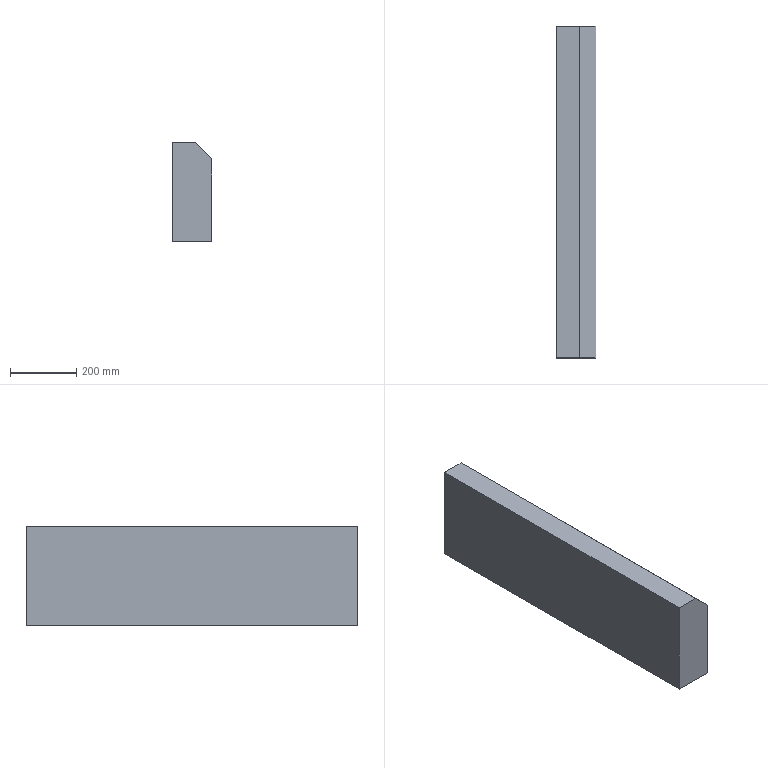Part | SolidWorks | features Chamfer 1, Extrusion 1 | 1 solid | 7 faces | box 120 x 1000 x 300 mm | volume 34750000 mm3 | plane 7
STEP:
#1=CARTESIAN_POINT('',(60.,500.,250.));
#2=VERTEX_POINT('',#1);
#3=CARTESIAN_POINT('',(60.,500.,0.));
#4=VERTEX_POINT('',#3);
#5=CARTESIAN_POINT('',(60.,500.,300.));
#6=DIRECTION('',(0.,0.,-1.));
#7=VECTOR('',#6,1000.);
#8=LINE('',#5,#7);
#9=EDGE_CURVE('',#2,#4,#8,.T.);
#10=ORIENTED_EDGE('',*,*,#9,.F.);
#11=CARTESIAN_POINT('',(60.,-500.,250.));
#12=VERTEX_POINT('',#11);
#13=CARTESIAN_POINT('',(60.,-500.,250.));
#14=DIRECTION('',(0.,-1.,0.));
#15=VECTOR('',#14,1000.);
#16=LINE('',#13,#15);
#17=EDGE_CURVE('',#2,#12,#16,.T.);
#18=ORIENTED_EDGE('',*,*,#17,.T.);
#19=CARTESIAN_POINT('',(60.,-500.,0.));
#20=VERTEX_POINT('',#19);
#21=CARTESIAN_POINT('',(60.,-500.,300.));
#22=DIRECTION('',(0.,0.,-1.));
#23=VECTOR('',#22,1000.);
#24=LINE('',#21,#23);
#25=EDGE_CURVE('',#12,#20,#24,.T.);
#26=ORIENTED_EDGE('',*,*,#25,.T.);
#27=CARTESIAN_POINT('',(60.,500.,0.));
#28=DIRECTION('',(0.,1.,0.));
#29=VECTOR('',#28,1000.);
#30=LINE('',#27,#29);
#31=EDGE_CURVE('',#20,#4,#30,.T.);
#32=ORIENTED_EDGE('',*,*,#31,.T.);
#33=EDGE_LOOP('',(#10,#18,#26,#32));
#34=FACE_OUTER_BOUND('',#33,.T.);
#35=CARTESIAN_POINT('',(60.,500.,300.));
#36=DIRECTION('',(-1.,0.,0.));
#37=DIRECTION('',(0.,-1.,0.));
#38=AXIS2_PLACEMENT_3D('',#35,#36,#37);
#39=PLANE('',#38);
#40=ADVANCED_FACE('',(#34),#39,.F.);
#41=CARTESIAN_POINT('',(10.,500.,300.));
#42=VERTEX_POINT('',#41);
#43=CARTESIAN_POINT('',(-60.,500.,300.));
#44=VERTEX_POINT('',#43);
#45=CARTESIAN_POINT('',(-60.,500.,300.));
#46=DIRECTION('',(-1.,0.,0.));
#47=VECTOR('',#46,1000.);
#48=LINE('',#45,#47);
#49=EDGE_CURVE('',#42,#44,#48,.T.);
#50=ORIENTED_EDGE('',*,*,#49,.F.);
#51=CARTESIAN_POINT('',(10.,500.,300.));
#52=DIRECTION('',(0.7071,0.,-0.7071));
#53=VECTOR('',#52,1000.);
#54=LINE('',#51,#53);
#55=EDGE_CURVE('',#42,#2,#54,.T.);
#56=ORIENTED_EDGE('',*,*,#55,.T.);
#57=ORIENTED_EDGE('',*,*,#9,.T.);
#58=CARTESIAN_POINT('',(-60.,500.,0.));
#59=VERTEX_POINT('',#58);
#60=CARTESIAN_POINT('',(-60.,500.,0.));
#61=DIRECTION('',(-1.,0.,0.));
#62=VECTOR('',#61,1000.);
#63=LINE('',#60,#62);
#64=EDGE_CURVE('',#4,#59,#63,.T.);
#65=ORIENTED_EDGE('',*,*,#64,.T.);
#66=CARTESIAN_POINT('',(-60.,500.,300.));
#67=DIRECTION('',(0.,0.,-1.));
#68=VECTOR('',#67,1000.);
#69=LINE('',#66,#68);
#70=EDGE_CURVE('',#44,#59,#69,.T.);
#71=ORIENTED_EDGE('',*,*,#70,.F.);
#72=EDGE_LOOP('',(#50,#56,#57,#65,#71));
#73=FACE_OUTER_BOUND('',#72,.T.);
#74=CARTESIAN_POINT('',(-60.,500.,300.));
#75=DIRECTION('',(0.,-1.,0.));
#76=DIRECTION('',(0.,0.,-1.));
#77=AXIS2_PLACEMENT_3D('',#74,#75,#76);
#78=PLANE('',#77);
#79=ADVANCED_FACE('',(#73),#78,.F.);
#80=CARTESIAN_POINT('',(-60.,-500.,0.));
#81=VERTEX_POINT('',#80);
#82=CARTESIAN_POINT('',(-60.,500.,0.));
#83=DIRECTION('',(0.,-1.,0.));
#84=VECTOR('',#83,1000.);
#85=LINE('',#82,#84);
#86=EDGE_CURVE('',#59,#81,#85,.T.);
#87=ORIENTED_EDGE('',*,*,#86,.T.);
#88=CARTESIAN_POINT('',(-60.,-500.,300.));
#89=VERTEX_POINT('',#88);
#90=CARTESIAN_POINT('',(-60.,-500.,300.));
#91=DIRECTION('',(0.,0.,-1.));
#92=VECTOR('',#91,1000.);
#93=LINE('',#90,#92);
#94=EDGE_CURVE('',#89,#81,#93,.T.);
#95=ORIENTED_EDGE('',*,*,#94,.F.);
#96=CARTESIAN_POINT('',(-60.,500.,300.));
#97=DIRECTION('',(0.,-1.,0.));
#98=VECTOR('',#97,1000.);
#99=LINE('',#96,#98);
#100=EDGE_CURVE('',#44,#89,#99,.T.);
#101=ORIENTED_EDGE('',*,*,#100,.F.);
#102=ORIENTED_EDGE('',*,*,#70,.T.);
#103=EDGE_LOOP('',(#87,#95,#101,#102));
#104=FACE_OUTER_BOUND('',#103,.T.);
#105=CARTESIAN_POINT('',(-60.,500.,300.));
#106=DIRECTION('',(1.,0.,0.));
#107=DIRECTION('',(0.,1.,0.));
#108=AXIS2_PLACEMENT_3D('',#105,#106,#107);
#109=PLANE('',#108);
#110=ADVANCED_FACE('',(#104),#109,.F.);
#111=ORIENTED_EDGE('',*,*,#25,.F.);
#112=CARTESIAN_POINT('',(10.,-500.,300.));
#113=VERTEX_POINT('',#112);
#114=CARTESIAN_POINT('',(10.,-500.,300.));
#115=DIRECTION('',(-0.7071,0.,0.7071));
#116=VECTOR('',#115,1000.);
#117=LINE('',#114,#116);
#118=EDGE_CURVE('',#12,#113,#117,.T.);
#119=ORIENTED_EDGE('',*,*,#118,.T.);
#120=CARTESIAN_POINT('',(-60.,-500.,300.));
#121=DIRECTION('',(1.,0.,0.));
#122=VECTOR('',#121,1000.);
#123=LINE('',#120,#122);
#124=EDGE_CURVE('',#89,#113,#123,.T.);
#125=ORIENTED_EDGE('',*,*,#124,.F.);
#126=ORIENTED_EDGE('',*,*,#94,.T.);
#127=CARTESIAN_POINT('',(-60.,-500.,0.));
#128=DIRECTION('',(1.,0.,0.));
#129=VECTOR('',#128,1000.);
#130=LINE('',#127,#129);
#131=EDGE_CURVE('',#81,#20,#130,.T.);
#132=ORIENTED_EDGE('',*,*,#131,.T.);
#133=EDGE_LOOP('',(#111,#119,#125,#126,#132));
#134=FACE_OUTER_BOUND('',#133,.T.);
#135=CARTESIAN_POINT('',(-60.,-500.,300.));
#136=DIRECTION('',(0.,1.,0.));
#137=DIRECTION('',(0.,0.,1.));
#138=AXIS2_PLACEMENT_3D('',#135,#136,#137);
#139=PLANE('',#138);
#140=ADVANCED_FACE('',(#134),#139,.F.);
#141=ORIENTED_EDGE('',*,*,#124,.T.);
#142=CARTESIAN_POINT('',(10.,500.,300.));
#143=DIRECTION('',(0.,1.,0.));
#144=VECTOR('',#143,1000.);
#145=LINE('',#142,#144);
#146=EDGE_CURVE('',#113,#42,#145,.T.);
#147=ORIENTED_EDGE('',*,*,#146,.T.);
#148=ORIENTED_EDGE('',*,*,#49,.T.);
#149=ORIENTED_EDGE('',*,*,#100,.T.);
#150=EDGE_LOOP('',(#141,#147,#148,#149));
#151=FACE_OUTER_BOUND('',#150,.T.);
#152=CARTESIAN_POINT('',(0.,0.,300.));
#153=DIRECTION('',(0.,0.,1.));
#154=DIRECTION('',(1.,0.,0.));
#155=AXIS2_PLACEMENT_3D('',#152,#153,#154);
#156=PLANE('',#155);
#157=ADVANCED_FACE('',(#151),#156,.T.);
#158=ORIENTED_EDGE('',*,*,#31,.F.);
#159=ORIENTED_EDGE('',*,*,#131,.F.);
#160=ORIENTED_EDGE('',*,*,#86,.F.);
#161=ORIENTED_EDGE('',*,*,#64,.F.);
#162=EDGE_LOOP('',(#158,#159,#160,#161));
#163=FACE_OUTER_BOUND('',#162,.T.);
#164=CARTESIAN_POINT('',(0.,0.,0.));
#165=DIRECTION('',(0.,0.,1.));
#166=DIRECTION('',(1.,0.,0.));
#167=AXIS2_PLACEMENT_3D('',#164,#165,#166);
#168=PLANE('',#167);
#169=ADVANCED_FACE('',(#163),#168,.F.);
#170=ORIENTED_EDGE('',*,*,#118,.F.);
#171=ORIENTED_EDGE('',*,*,#17,.F.);
#172=ORIENTED_EDGE('',*,*,#55,.F.);
#173=ORIENTED_EDGE('',*,*,#146,.F.);
#174=EDGE_LOOP('',(#170,#171,#172,#173));
#175=FACE_OUTER_BOUND('',#174,.T.);
#176=CARTESIAN_POINT('',(10.,0.,300.));
#177=DIRECTION('',(0.7071,0.,0.7071));
#178=DIRECTION('',(0.,-1.,0.));
#179=AXIS2_PLACEMENT_3D('',#176,#177,#178);
#180=PLANE('',#179);
#181=ADVANCED_FACE('',(#175),#180,.T.);
#182=CLOSED_SHELL('',(#40,#79,#110,#140,#157,#169,#181));
#183=MANIFOLD_SOLID_BREP('',#182);
#184=CARTESIAN_POINT('',(0.,0.,0.));
#185=DIRECTION('',(0.,0.,1.));
#186=DIRECTION('',(1.,0.,0.));
#187=AXIS2_PLACEMENT_3D('',#184,#185,#186);
#188=(LENGTH_UNIT()NAMED_UNIT(*)SI_UNIT(.MILLI.,.METRE.));
#189=UNCERTAINTY_MEASURE_WITH_UNIT(LENGTH_MEASURE(0.00001),#188,'','');
#190=(NAMED_UNIT(*)PLANE_ANGLE_UNIT()SI_UNIT($,.RADIAN.));
#191=(NAMED_UNIT(*)SI_UNIT($,.STERADIAN.)SOLID_ANGLE_UNIT());
#192=(GEOMETRIC_REPRESENTATION_CONTEXT(3)GLOBAL_UNCERTAINTY_ASSIGNED_CONTEXT((#189))GLOBAL_UNIT_ASSIGNED_CONTEXT((#188,#190,#191))REPRESENTATION_CONTEXT('',''));
#193=ADVANCED_BREP_SHAPE_REPRESENTATION('',(#183,#187),#192);